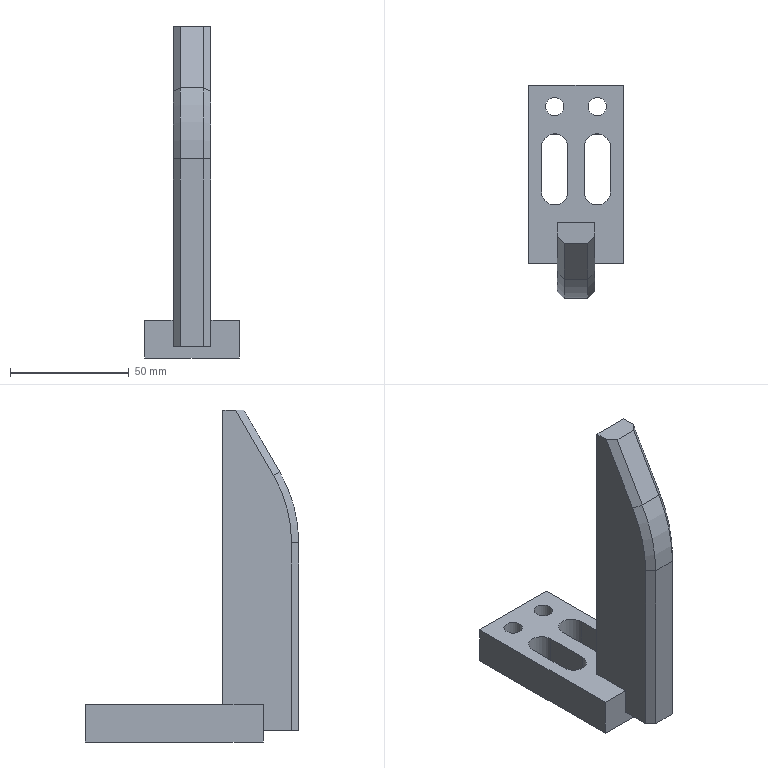Part | NX | features solid 2 | 1 solid | 30 faces | box 40 x 90 x 140 mm | volume 93861 mm3 | plane 21 | cylinder 7 | cone 2 | commonest cylinder face diameters 11 x4 7.8 x2 120 x1
STEP:
#1=CARTESIAN_POINT('',(599.5,194.,-54.));
#2=VERTEX_POINT('',#1);
#3=CARTESIAN_POINT('',(588.5,194.,-54.));
#4=VERTEX_POINT('',#3);
#5=CARTESIAN_POINT('',(594.,194.,-54.));
#6=DIRECTION('',(0.,0.,1.));
#7=DIRECTION('',(0.,-1.,0.));
#8=AXIS2_PLACEMENT_3D('',#5,#6,#7);
#9=CIRCLE('',#8,5.5);
#10=EDGE_CURVE('',#2,#4,#9,.T.);
#11=ORIENTED_EDGE('',*,*,#10,.F.);
#12=CARTESIAN_POINT('',(599.5,175.,-54.));
#13=VERTEX_POINT('',#12);
#14=CARTESIAN_POINT('',(599.5,194.,-54.));
#15=DIRECTION('',(0.,-1.,0.));
#16=VECTOR('',#15,1000.);
#17=LINE('',#14,#16);
#18=EDGE_CURVE('',#2,#13,#17,.T.);
#19=ORIENTED_EDGE('',*,*,#18,.T.);
#20=CARTESIAN_POINT('',(588.5,175.,-54.));
#21=VERTEX_POINT('',#20);
#22=CARTESIAN_POINT('',(594.,175.,-54.));
#23=DIRECTION('',(0.,0.,1.));
#24=DIRECTION('',(0.,-1.,0.));
#25=AXIS2_PLACEMENT_3D('',#22,#23,#24);
#26=CIRCLE('',#25,5.5);
#27=EDGE_CURVE('',#21,#13,#26,.T.);
#28=ORIENTED_EDGE('',*,*,#27,.F.);
#29=CARTESIAN_POINT('',(588.5,194.,-54.));
#30=DIRECTION('',(0.,-1.,0.));
#31=VECTOR('',#30,1000.);
#32=LINE('',#29,#31);
#33=EDGE_CURVE('',#4,#21,#32,.T.);
#34=ORIENTED_EDGE('',*,*,#33,.F.);
#35=EDGE_LOOP('',(#11,#19,#28,#34));
#36=FACE_BOUND('',#35,.T.);
#37=CARTESIAN_POINT('',(576.,207.1,-54.));
#38=VERTEX_POINT('',#37);
#39=CARTESIAN_POINT('',(576.,211.,-54.));
#40=DIRECTION('',(0.,0.,1.));
#41=DIRECTION('',(0.,-1.,0.));
#42=AXIS2_PLACEMENT_3D('',#39,#40,#41);
#43=CIRCLE('',#42,3.9);
#44=EDGE_CURVE('',#38,#38,#43,.T.);
#45=ORIENTED_EDGE('',*,*,#44,.F.);
#46=EDGE_LOOP('',(#45));
#47=FACE_BOUND('',#46,.T.);
#48=CARTESIAN_POINT('',(594.,207.1,-54.));
#49=VERTEX_POINT('',#48);
#50=CARTESIAN_POINT('',(594.,211.,-54.));
#51=DIRECTION('',(0.,0.,1.));
#52=DIRECTION('',(0.,-1.,0.));
#53=AXIS2_PLACEMENT_3D('',#50,#51,#52);
#54=CIRCLE('',#53,3.9);
#55=EDGE_CURVE('',#49,#49,#54,.T.);
#56=ORIENTED_EDGE('',*,*,#55,.F.);
#57=EDGE_LOOP('',(#56));
#58=FACE_BOUND('',#57,.T.);
#59=CARTESIAN_POINT('',(581.5,194.,-54.));
#60=VERTEX_POINT('',#59);
#61=CARTESIAN_POINT('',(581.5,175.,-54.));
#62=VERTEX_POINT('',#61);
#63=CARTESIAN_POINT('',(581.5,194.,-54.));
#64=DIRECTION('',(0.,-1.,0.));
#65=VECTOR('',#64,1000.);
#66=LINE('',#63,#65);
#67=EDGE_CURVE('',#60,#62,#66,.T.);
#68=ORIENTED_EDGE('',*,*,#67,.T.);
#69=CARTESIAN_POINT('',(570.5,175.,-54.));
#70=VERTEX_POINT('',#69);
#71=CARTESIAN_POINT('',(576.,175.,-54.));
#72=DIRECTION('',(0.,0.,1.));
#73=DIRECTION('',(0.,-1.,0.));
#74=AXIS2_PLACEMENT_3D('',#71,#72,#73);
#75=CIRCLE('',#74,5.5);
#76=EDGE_CURVE('',#70,#62,#75,.T.);
#77=ORIENTED_EDGE('',*,*,#76,.F.);
#78=CARTESIAN_POINT('',(570.5,194.,-54.));
#79=VERTEX_POINT('',#78);
#80=CARTESIAN_POINT('',(570.5,194.,-54.));
#81=DIRECTION('',(0.,-1.,0.));
#82=VECTOR('',#81,1000.);
#83=LINE('',#80,#82);
#84=EDGE_CURVE('',#79,#70,#83,.T.);
#85=ORIENTED_EDGE('',*,*,#84,.F.);
#86=CARTESIAN_POINT('',(576.,194.,-54.));
#87=DIRECTION('',(0.,0.,1.));
#88=DIRECTION('',(0.,-1.,0.));
#89=AXIS2_PLACEMENT_3D('',#86,#87,#88);
#90=CIRCLE('',#89,5.5);
#91=EDGE_CURVE('',#60,#79,#90,.T.);
#92=ORIENTED_EDGE('',*,*,#91,.F.);
#93=EDGE_LOOP('',(#68,#77,#85,#92));
#94=FACE_BOUND('',#93,.T.);
#95=CARTESIAN_POINT('',(593.,162.,-54.));
#96=VERTEX_POINT('',#95);
#97=CARTESIAN_POINT('',(577.,162.,-54.));
#98=VERTEX_POINT('',#97);
#99=CARTESIAN_POINT('',(677.,162.,-54.));
#100=DIRECTION('',(-1.,0.,0.));
#101=VECTOR('',#100,1000.);
#102=LINE('',#99,#101);
#103=EDGE_CURVE('',#96,#98,#102,.T.);
#104=ORIENTED_EDGE('',*,*,#103,.F.);
#105=CARTESIAN_POINT('',(593.,145.,-54.));
#106=VERTEX_POINT('',#105);
#107=CARTESIAN_POINT('',(593.,162.,-54.));
#108=DIRECTION('',(0.,1.,0.));
#109=VECTOR('',#108,1000.);
#110=LINE('',#107,#109);
#111=EDGE_CURVE('',#106,#96,#110,.T.);
#112=ORIENTED_EDGE('',*,*,#111,.F.);
#113=CARTESIAN_POINT('',(605.,145.,-54.));
#114=VERTEX_POINT('',#113);
#115=CARTESIAN_POINT('',(585.,145.,-54.));
#116=DIRECTION('',(1.,0.,0.));
#117=VECTOR('',#116,1000.);
#118=LINE('',#115,#117);
#119=EDGE_CURVE('',#106,#114,#118,.T.);
#120=ORIENTED_EDGE('',*,*,#119,.T.);
#121=CARTESIAN_POINT('',(605.,220.,-54.));
#122=VERTEX_POINT('',#121);
#123=CARTESIAN_POINT('',(605.,182.5,-54.));
#124=DIRECTION('',(0.,1.,0.));
#125=VECTOR('',#124,1000.);
#126=LINE('',#123,#125);
#127=EDGE_CURVE('',#114,#122,#126,.T.);
#128=ORIENTED_EDGE('',*,*,#127,.T.);
#129=CARTESIAN_POINT('',(565.,220.,-54.));
#130=VERTEX_POINT('',#129);
#131=CARTESIAN_POINT('',(585.,220.,-54.));
#132=DIRECTION('',(-1.,0.,0.));
#133=VECTOR('',#132,1000.);
#134=LINE('',#131,#133);
#135=EDGE_CURVE('',#122,#130,#134,.T.);
#136=ORIENTED_EDGE('',*,*,#135,.T.);
#137=CARTESIAN_POINT('',(565.,145.,-54.));
#138=VERTEX_POINT('',#137);
#139=CARTESIAN_POINT('',(565.,182.5,-54.));
#140=DIRECTION('',(0.,-1.,0.));
#141=VECTOR('',#140,1000.);
#142=LINE('',#139,#141);
#143=EDGE_CURVE('',#130,#138,#142,.T.);
#144=ORIENTED_EDGE('',*,*,#143,.T.);
#145=CARTESIAN_POINT('',(577.,145.,-54.));
#146=VERTEX_POINT('',#145);
#147=CARTESIAN_POINT('',(585.,145.,-54.));
#148=DIRECTION('',(1.,0.,0.));
#149=VECTOR('',#148,1000.);
#150=LINE('',#147,#149);
#151=EDGE_CURVE('',#138,#146,#150,.T.);
#152=ORIENTED_EDGE('',*,*,#151,.T.);
#153=CARTESIAN_POINT('',(577.,130.,-54.));
#154=DIRECTION('',(0.,1.,0.));
#155=VECTOR('',#154,1000.);
#156=LINE('',#153,#155);
#157=EDGE_CURVE('',#146,#98,#156,.T.);
#158=ORIENTED_EDGE('',*,*,#157,.T.);
#159=EDGE_LOOP('',(#104,#112,#120,#128,#136,#144,#152,#158));
#160=FACE_BOUND('',#159,.T.);
#161=CARTESIAN_POINT('',(585.,182.5,-54.));
#162=DIRECTION('',(0.,0.,1.));
#163=DIRECTION('',(0.,-1.,0.));
#164=AXIS2_PLACEMENT_3D('',#161,#162,#163);
#165=PLANE('',#164);
#166=ADVANCED_FACE('',(#36,#47,#58,#94,#160),#165,.T.);
#167=ORIENTED_EDGE('',*,*,#151,.F.);
#168=CARTESIAN_POINT('',(565.,145.,-70.));
#169=VERTEX_POINT('',#168);
#170=CARTESIAN_POINT('',(565.,145.,-70.));
#171=DIRECTION('',(0.,0.,1.));
#172=VECTOR('',#171,1000.);
#173=LINE('',#170,#172);
#174=EDGE_CURVE('',#169,#138,#173,.T.);
#175=ORIENTED_EDGE('',*,*,#174,.F.);
#176=CARTESIAN_POINT('',(605.,145.,-70.));
#177=VERTEX_POINT('',#176);
#178=CARTESIAN_POINT('',(585.,145.,-70.));
#179=DIRECTION('',(-1.,0.,0.));
#180=VECTOR('',#179,1000.);
#181=LINE('',#178,#180);
#182=EDGE_CURVE('',#177,#169,#181,.T.);
#183=ORIENTED_EDGE('',*,*,#182,.F.);
#184=CARTESIAN_POINT('',(605.,145.,-70.));
#185=DIRECTION('',(0.,0.,1.));
#186=VECTOR('',#185,1000.);
#187=LINE('',#184,#186);
#188=EDGE_CURVE('',#177,#114,#187,.T.);
#189=ORIENTED_EDGE('',*,*,#188,.T.);
#190=ORIENTED_EDGE('',*,*,#119,.F.);
#191=CARTESIAN_POINT('',(593.,145.,-65.));
#192=VERTEX_POINT('',#191);
#193=CARTESIAN_POINT('',(593.,145.,35.));
#194=DIRECTION('',(0.,0.,1.));
#195=VECTOR('',#194,1000.);
#196=LINE('',#193,#195);
#197=EDGE_CURVE('',#192,#106,#196,.T.);
#198=ORIENTED_EDGE('',*,*,#197,.F.);
#199=CARTESIAN_POINT('',(577.,145.,-65.));
#200=VERTEX_POINT('',#199);
#201=CARTESIAN_POINT('',(677.,145.,-65.));
#202=DIRECTION('',(-1.,0.,0.));
#203=VECTOR('',#202,1000.);
#204=LINE('',#201,#203);
#205=EDGE_CURVE('',#192,#200,#204,.T.);
#206=ORIENTED_EDGE('',*,*,#205,.T.);
#207=CARTESIAN_POINT('',(577.,145.,-75.));
#208=DIRECTION('',(0.,0.,1.));
#209=VECTOR('',#208,1000.);
#210=LINE('',#207,#209);
#211=EDGE_CURVE('',#200,#146,#210,.T.);
#212=ORIENTED_EDGE('',*,*,#211,.T.);
#213=EDGE_LOOP('',(#167,#175,#183,#189,#190,#198,#206,#212));
#214=FACE_BOUND('',#213,.T.);
#215=CARTESIAN_POINT('',(585.,145.,-70.));
#216=DIRECTION('',(0.,-1.,0.));
#217=DIRECTION('',(0.,0.,-1.));
#218=AXIS2_PLACEMENT_3D('',#215,#216,#217);
#219=PLANE('',#218);
#220=ADVANCED_FACE('',(#214),#219,.T.);
#221=CARTESIAN_POINT('',(581.5,194.,-70.));
#222=VERTEX_POINT('',#221);
#223=CARTESIAN_POINT('',(581.5,194.,-154.));
#224=DIRECTION('',(0.,0.,1.));
#225=VECTOR('',#224,1000.);
#226=LINE('',#223,#225);
#227=EDGE_CURVE('',#222,#60,#226,.T.);
#228=ORIENTED_EDGE('',*,*,#227,.T.);
#229=ORIENTED_EDGE('',*,*,#91,.T.);
#230=CARTESIAN_POINT('',(570.5,194.,-70.));
#231=VERTEX_POINT('',#230);
#232=CARTESIAN_POINT('',(570.5,194.,-154.));
#233=DIRECTION('',(0.,0.,1.));
#234=VECTOR('',#233,1000.);
#235=LINE('',#232,#234);
#236=EDGE_CURVE('',#231,#79,#235,.T.);
#237=ORIENTED_EDGE('',*,*,#236,.F.);
#238=CARTESIAN_POINT('',(576.,194.,-70.));
#239=DIRECTION('',(0.,0.,1.));
#240=DIRECTION('',(0.,-1.,0.));
#241=AXIS2_PLACEMENT_3D('',#238,#239,#240);
#242=CIRCLE('',#241,5.5);
#243=EDGE_CURVE('',#222,#231,#242,.T.);
#244=ORIENTED_EDGE('',*,*,#243,.F.);
#245=EDGE_LOOP('',(#228,#229,#237,#244));
#246=FACE_BOUND('',#245,.T.);
#247=CARTESIAN_POINT('',(576.,194.,-54.));
#248=DIRECTION('',(0.,0.,-1.));
#249=DIRECTION('',(0.,1.,0.));
#250=AXIS2_PLACEMENT_3D('',#247,#248,#249);
#251=CYLINDRICAL_SURFACE('',#250,5.5);
#252=ADVANCED_FACE('',(#246),#251,.F.);
#253=CARTESIAN_POINT('',(581.5,175.,-70.));
#254=VERTEX_POINT('',#253);
#255=CARTESIAN_POINT('',(581.5,182.5,-70.));
#256=DIRECTION('',(0.,1.,0.));
#257=VECTOR('',#256,1000.);
#258=LINE('',#255,#257);
#259=EDGE_CURVE('',#254,#222,#258,.T.);
#260=ORIENTED_EDGE('',*,*,#259,.T.);
#261=ORIENTED_EDGE('',*,*,#243,.T.);
#262=CARTESIAN_POINT('',(570.5,175.,-70.));
#263=VERTEX_POINT('',#262);
#264=CARTESIAN_POINT('',(570.5,182.5,-70.));
#265=DIRECTION('',(0.,1.,0.));
#266=VECTOR('',#265,1000.);
#267=LINE('',#264,#266);
#268=EDGE_CURVE('',#263,#231,#267,.T.);
#269=ORIENTED_EDGE('',*,*,#268,.F.);
#270=CARTESIAN_POINT('',(576.,175.,-70.));
#271=DIRECTION('',(0.,0.,1.));
#272=DIRECTION('',(0.,-1.,0.));
#273=AXIS2_PLACEMENT_3D('',#270,#271,#272);
#274=CIRCLE('',#273,5.5);
#275=EDGE_CURVE('',#263,#254,#274,.T.);
#276=ORIENTED_EDGE('',*,*,#275,.T.);
#277=EDGE_LOOP('',(#260,#261,#269,#276));
#278=FACE_BOUND('',#277,.T.);
#279=CARTESIAN_POINT('',(565.,220.,-70.));
#280=VERTEX_POINT('',#279);
#281=CARTESIAN_POINT('',(605.,220.,-70.));
#282=VERTEX_POINT('',#281);
#283=CARTESIAN_POINT('',(585.,220.,-70.));
#284=DIRECTION('',(1.,0.,0.));
#285=VECTOR('',#284,1000.);
#286=LINE('',#283,#285);
#287=EDGE_CURVE('',#280,#282,#286,.T.);
#288=ORIENTED_EDGE('',*,*,#287,.T.);
#289=CARTESIAN_POINT('',(605.,182.5,-70.));
#290=DIRECTION('',(0.,-1.,0.));
#291=VECTOR('',#290,1000.);
#292=LINE('',#289,#291);
#293=EDGE_CURVE('',#282,#177,#292,.T.);
#294=ORIENTED_EDGE('',*,*,#293,.T.);
#295=ORIENTED_EDGE('',*,*,#182,.T.);
#296=CARTESIAN_POINT('',(565.,182.5,-70.));
#297=DIRECTION('',(0.,1.,0.));
#298=VECTOR('',#297,1000.);
#299=LINE('',#296,#298);
#300=EDGE_CURVE('',#169,#280,#299,.T.);
#301=ORIENTED_EDGE('',*,*,#300,.T.);
#302=EDGE_LOOP('',(#288,#294,#295,#301));
#303=FACE_BOUND('',#302,.T.);
#304=CARTESIAN_POINT('',(594.,207.1,-70.));
#305=VERTEX_POINT('',#304);
#306=CARTESIAN_POINT('',(594.,211.,-70.));
#307=DIRECTION('',(0.,0.,1.));
#308=DIRECTION('',(0.,-1.,0.));
#309=AXIS2_PLACEMENT_3D('',#306,#307,#308);
#310=CIRCLE('',#309,3.9);
#311=EDGE_CURVE('',#305,#305,#310,.T.);
#312=ORIENTED_EDGE('',*,*,#311,.T.);
#313=EDGE_LOOP('',(#312));
#314=FACE_BOUND('',#313,.T.);
#315=CARTESIAN_POINT('',(576.,207.1,-70.));
#316=VERTEX_POINT('',#315);
#317=CARTESIAN_POINT('',(576.,211.,-70.));
#318=DIRECTION('',(0.,0.,1.));
#319=DIRECTION('',(0.,-1.,0.));
#320=AXIS2_PLACEMENT_3D('',#317,#318,#319);
#321=CIRCLE('',#320,3.9);
#322=EDGE_CURVE('',#316,#316,#321,.T.);
#323=ORIENTED_EDGE('',*,*,#322,.T.);
#324=EDGE_LOOP('',(#323));
#325=FACE_BOUND('',#324,.T.);
#326=CARTESIAN_POINT('',(588.5,175.,-70.));
#327=VERTEX_POINT('',#326);
#328=CARTESIAN_POINT('',(599.5,175.,-70.));
#329=VERTEX_POINT('',#328);
#330=CARTESIAN_POINT('',(594.,175.,-70.));
#331=DIRECTION('',(0.,0.,1.));
#332=DIRECTION('',(0.,-1.,0.));
#333=AXIS2_PLACEMENT_3D('',#330,#331,#332);
#334=CIRCLE('',#333,5.5);
#335=EDGE_CURVE('',#327,#329,#334,.T.);
#336=ORIENTED_EDGE('',*,*,#335,.T.);
#337=CARTESIAN_POINT('',(599.5,194.,-70.));
#338=VERTEX_POINT('',#337);
#339=CARTESIAN_POINT('',(599.5,182.5,-70.));
#340=DIRECTION('',(0.,1.,0.));
#341=VECTOR('',#340,1000.);
#342=LINE('',#339,#341);
#343=EDGE_CURVE('',#329,#338,#342,.T.);
#344=ORIENTED_EDGE('',*,*,#343,.T.);
#345=CARTESIAN_POINT('',(588.5,194.,-70.));
#346=VERTEX_POINT('',#345);
#347=CARTESIAN_POINT('',(594.,194.,-70.));
#348=DIRECTION('',(0.,0.,1.));
#349=DIRECTION('',(0.,-1.,0.));
#350=AXIS2_PLACEMENT_3D('',#347,#348,#349);
#351=CIRCLE('',#350,5.5);
#352=EDGE_CURVE('',#338,#346,#351,.T.);
#353=ORIENTED_EDGE('',*,*,#352,.T.);
#354=CARTESIAN_POINT('',(588.5,182.5,-70.));
#355=DIRECTION('',(0.,1.,0.));
#356=VECTOR('',#355,1000.);
#357=LINE('',#354,#356);
#358=EDGE_CURVE('',#327,#346,#357,.T.);
#359=ORIENTED_EDGE('',*,*,#358,.F.);
#360=EDGE_LOOP('',(#336,#344,#353,#359));
#361=FACE_BOUND('',#360,.T.);
#362=CARTESIAN_POINT('',(585.,182.5,-70.));
#363=DIRECTION('',(0.,0.,-1.));
#364=DIRECTION('',(0.,1.,0.));
#365=AXIS2_PLACEMENT_3D('',#362,#363,#364);
#366=PLANE('',#365);
#367=ADVANCED_FACE('',(#278,#303,#314,#325,#361),#366,.T.);
#368=CARTESIAN_POINT('',(588.5,175.,-154.));
#369=DIRECTION('',(0.,0.,1.));
#370=VECTOR('',#369,1000.);
#371=LINE('',#368,#370);
#372=EDGE_CURVE('',#327,#21,#371,.T.);
#373=ORIENTED_EDGE('',*,*,#372,.T.);
#374=ORIENTED_EDGE('',*,*,#27,.T.);
#375=CARTESIAN_POINT('',(599.5,175.,-154.));
#376=DIRECTION('',(0.,0.,1.));
#377=VECTOR('',#376,1000.);
#378=LINE('',#375,#377);
#379=EDGE_CURVE('',#329,#13,#378,.T.);
#380=ORIENTED_EDGE('',*,*,#379,.F.);
#381=ORIENTED_EDGE('',*,*,#335,.F.);
#382=EDGE_LOOP('',(#373,#374,#380,#381));
#383=FACE_BOUND('',#382,.T.);
#384=CARTESIAN_POINT('',(594.,175.,-54.));
#385=DIRECTION('',(0.,0.,-1.));
#386=DIRECTION('',(0.,1.,0.));
#387=AXIS2_PLACEMENT_3D('',#384,#385,#386);
#388=CYLINDRICAL_SURFACE('',#387,5.5);
#389=ADVANCED_FACE('',(#383),#388,.F.);
#390=CARTESIAN_POINT('',(565.,220.,-70.));
#391=DIRECTION('',(0.,0.,1.));
#392=VECTOR('',#391,1000.);
#393=LINE('',#390,#392);
#394=EDGE_CURVE('',#280,#130,#393,.T.);
#395=ORIENTED_EDGE('',*,*,#394,.F.);
#396=ORIENTED_EDGE('',*,*,#300,.F.);
#397=ORIENTED_EDGE('',*,*,#174,.T.);
#398=ORIENTED_EDGE('',*,*,#143,.F.);
#399=EDGE_LOOP('',(#395,#396,#397,#398));
#400=FACE_BOUND('',#399,.T.);
#401=CARTESIAN_POINT('',(565.,182.5,-70.));
#402=DIRECTION('',(-1.,0.,0.));
#403=DIRECTION('',(0.,0.,1.));
#404=AXIS2_PLACEMENT_3D('',#401,#402,#403);
#405=PLANE('',#404);
#406=ADVANCED_FACE('',(#400),#405,.T.);
#407=ORIENTED_EDGE('',*,*,#188,.F.);
#408=ORIENTED_EDGE('',*,*,#293,.F.);
#409=CARTESIAN_POINT('',(605.,220.,-70.));
#410=DIRECTION('',(0.,0.,1.));
#411=VECTOR('',#410,1000.);
#412=LINE('',#409,#411);
#413=EDGE_CURVE('',#282,#122,#412,.T.);
#414=ORIENTED_EDGE('',*,*,#413,.T.);
#415=ORIENTED_EDGE('',*,*,#127,.F.);
#416=EDGE_LOOP('',(#407,#408,#414,#415));
#417=FACE_BOUND('',#416,.T.);
#418=CARTESIAN_POINT('',(605.,182.5,-70.));
#419=DIRECTION('',(1.,0.,0.));
#420=DIRECTION('',(0.,0.,-1.));
#421=AXIS2_PLACEMENT_3D('',#418,#419,#420);
#422=PLANE('',#421);
#423=ADVANCED_FACE('',(#417),#422,.T.);
#424=ORIENTED_EDGE('',*,*,#287,.F.);
#425=ORIENTED_EDGE('',*,*,#394,.T.);
#426=ORIENTED_EDGE('',*,*,#135,.F.);
#427=ORIENTED_EDGE('',*,*,#413,.F.);
#428=EDGE_LOOP('',(#424,#425,#426,#427));
#429=FACE_BOUND('',#428,.T.);
#430=CARTESIAN_POINT('',(585.,220.,-70.));
#431=DIRECTION('',(0.,1.,0.));
#432=DIRECTION('',(0.,0.,1.));
#433=AXIS2_PLACEMENT_3D('',#430,#431,#432);
#434=PLANE('',#433);
#435=ADVANCED_FACE('',(#429),#434,.T.);
#436=ORIENTED_EDGE('',*,*,#275,.F.);
#437=CARTESIAN_POINT('',(570.5,175.,-154.));
#438=DIRECTION('',(0.,0.,1.));
#439=VECTOR('',#438,1000.);
#440=LINE('',#437,#439);
#441=EDGE_CURVE('',#263,#70,#440,.T.);
#442=ORIENTED_EDGE('',*,*,#441,.T.);
#443=ORIENTED_EDGE('',*,*,#76,.T.);
#444=CARTESIAN_POINT('',(581.5,175.,-154.));
#445=DIRECTION('',(0.,0.,1.));
#446=VECTOR('',#445,1000.);
#447=LINE('',#444,#446);
#448=EDGE_CURVE('',#254,#62,#447,.T.);
#449=ORIENTED_EDGE('',*,*,#448,.F.);
#450=EDGE_LOOP('',(#436,#442,#443,#449));
#451=FACE_BOUND('',#450,.T.);
#452=CARTESIAN_POINT('',(576.,175.,-54.));
#453=DIRECTION('',(0.,0.,-1.));
#454=DIRECTION('',(0.,1.,0.));
#455=AXIS2_PLACEMENT_3D('',#452,#453,#454);
#456=CYLINDRICAL_SURFACE('',#455,5.5);
#457=ADVANCED_FACE('',(#451),#456,.F.);
#458=ORIENTED_EDGE('',*,*,#352,.F.);
#459=CARTESIAN_POINT('',(599.5,194.,-154.));
#460=DIRECTION('',(0.,0.,1.));
#461=VECTOR('',#460,1000.);
#462=LINE('',#459,#461);
#463=EDGE_CURVE('',#338,#2,#462,.T.);
#464=ORIENTED_EDGE('',*,*,#463,.T.);
#465=ORIENTED_EDGE('',*,*,#10,.T.);
#466=CARTESIAN_POINT('',(588.5,194.,-154.));
#467=DIRECTION('',(0.,0.,1.));
#468=VECTOR('',#467,1000.);
#469=LINE('',#466,#468);
#470=EDGE_CURVE('',#346,#4,#469,.T.);
#471=ORIENTED_EDGE('',*,*,#470,.F.);
#472=EDGE_LOOP('',(#458,#464,#465,#471));
#473=FACE_BOUND('',#472,.T.);
#474=CARTESIAN_POINT('',(594.,194.,-54.));
#475=DIRECTION('',(0.,0.,-1.));
#476=DIRECTION('',(0.,1.,0.));
#477=AXIS2_PLACEMENT_3D('',#474,#475,#476);
#478=CYLINDRICAL_SURFACE('',#477,5.5);
#479=ADVANCED_FACE('',(#473),#478,.F.);
#480=ORIENTED_EDGE('',*,*,#311,.F.);
#481=EDGE_LOOP('',(#480));
#482=FACE_BOUND('',#481,.T.);
#483=ORIENTED_EDGE('',*,*,#55,.T.);
#484=EDGE_LOOP('',(#483));
#485=FACE_BOUND('',#484,.T.);
#486=CARTESIAN_POINT('',(594.,211.,-54.));
#487=DIRECTION('',(0.,0.,-1.));
#488=DIRECTION('',(0.,1.,0.));
#489=AXIS2_PLACEMENT_3D('',#486,#487,#488);
#490=CYLINDRICAL_SURFACE('',#489,3.9);
#491=ADVANCED_FACE('',(#482,#485),#490,.F.);
#492=ORIENTED_EDGE('',*,*,#322,.F.);
#493=EDGE_LOOP('',(#492));
#494=FACE_BOUND('',#493,.T.);
#495=ORIENTED_EDGE('',*,*,#44,.T.);
#496=EDGE_LOOP('',(#495));
#497=FACE_BOUND('',#496,.T.);
#498=CARTESIAN_POINT('',(576.,211.,-54.));
#499=DIRECTION('',(0.,0.,-1.));
#500=DIRECTION('',(0.,1.,0.));
#501=AXIS2_PLACEMENT_3D('',#498,#499,#500);
#502=CYLINDRICAL_SURFACE('',#501,3.9);
#503=ADVANCED_FACE('',(#494,#497),#502,.F.);
#504=ORIENTED_EDGE('',*,*,#343,.F.);
#505=ORIENTED_EDGE('',*,*,#379,.T.);
#506=ORIENTED_EDGE('',*,*,#18,.F.);
#507=ORIENTED_EDGE('',*,*,#463,.F.);
#508=EDGE_LOOP('',(#504,#505,#506,#507));
#509=FACE_BOUND('',#508,.T.);
#510=CARTESIAN_POINT('',(599.5,194.,-154.));
#511=DIRECTION('',(1.,0.,0.));
#512=DIRECTION('',(0.,0.,-1.));
#513=AXIS2_PLACEMENT_3D('',#510,#511,#512);
#514=PLANE('',#513);
#515=ADVANCED_FACE('',(#509),#514,.F.);
#516=ORIENTED_EDGE('',*,*,#372,.F.);
#517=ORIENTED_EDGE('',*,*,#358,.T.);
#518=ORIENTED_EDGE('',*,*,#470,.T.);
#519=ORIENTED_EDGE('',*,*,#33,.T.);
#520=EDGE_LOOP('',(#516,#517,#518,#519));
#521=FACE_BOUND('',#520,.T.);
#522=CARTESIAN_POINT('',(588.5,194.,-154.));
#523=DIRECTION('',(1.,0.,0.));
#524=DIRECTION('',(0.,0.,-1.));
#525=AXIS2_PLACEMENT_3D('',#522,#523,#524);
#526=PLANE('',#525);
#527=ADVANCED_FACE('',(#521),#526,.T.);
#528=ORIENTED_EDGE('',*,*,#441,.F.);
#529=ORIENTED_EDGE('',*,*,#268,.T.);
#530=ORIENTED_EDGE('',*,*,#236,.T.);
#531=ORIENTED_EDGE('',*,*,#84,.T.);
#532=EDGE_LOOP('',(#528,#529,#530,#531));
#533=FACE_BOUND('',#532,.T.);
#534=CARTESIAN_POINT('',(570.5,194.,-154.));
#535=DIRECTION('',(1.,0.,0.));
#536=DIRECTION('',(0.,0.,-1.));
#537=AXIS2_PLACEMENT_3D('',#534,#535,#536);
#538=PLANE('',#537);
#539=ADVANCED_FACE('',(#533),#538,.T.);
#540=ORIENTED_EDGE('',*,*,#259,.F.);
#541=ORIENTED_EDGE('',*,*,#448,.T.);
#542=ORIENTED_EDGE('',*,*,#67,.F.);
#543=ORIENTED_EDGE('',*,*,#227,.F.);
#544=EDGE_LOOP('',(#540,#541,#542,#543));
#545=FACE_BOUND('',#544,.T.);
#546=CARTESIAN_POINT('',(581.5,194.,-154.));
#547=DIRECTION('',(1.,0.,0.));
#548=DIRECTION('',(0.,0.,-1.));
#549=AXIS2_PLACEMENT_3D('',#546,#547,#548);
#550=PLANE('',#549);
#551=ADVANCED_FACE('',(#545),#550,.F.);
#552=ORIENTED_EDGE('',*,*,#211,.F.);
#553=CARTESIAN_POINT('',(577.,133.,-65.));
#554=VERTEX_POINT('',#553);
#555=CARTESIAN_POINT('',(577.,130.,-65.));
#556=DIRECTION('',(0.,1.,0.));
#557=VECTOR('',#556,1000.);
#558=LINE('',#555,#557);
#559=EDGE_CURVE('',#554,#200,#558,.T.);
#560=ORIENTED_EDGE('',*,*,#559,.F.);
#561=CARTESIAN_POINT('',(577.,133.,13.923));
#562=VERTEX_POINT('',#561);
#563=CARTESIAN_POINT('',(577.,133.,35.));
#564=DIRECTION('',(0.,0.,-1.));
#565=VECTOR('',#564,1000.);
#566=LINE('',#563,#565);
#567=EDGE_CURVE('',#562,#554,#566,.T.);
#568=ORIENTED_EDGE('',*,*,#567,.F.);
#569=CARTESIAN_POINT('',(577.,140.637,42.423));
#570=VERTEX_POINT('',#569);
#571=CARTESIAN_POINT('',(577.,190.,13.923));
#572=DIRECTION('',(1.,0.,0.));
#573=DIRECTION('',(0.,0.,1.));
#574=AXIS2_PLACEMENT_3D('',#571,#572,#573);
#575=CIRCLE('',#574,57.);
#576=EDGE_CURVE('',#570,#562,#575,.T.);
#577=ORIENTED_EDGE('',*,*,#576,.F.);
#578=CARTESIAN_POINT('',(577.,156.558,70.));
#579=VERTEX_POINT('',#578);
#580=CARTESIAN_POINT('',(577.,149.919,58.5));
#581=DIRECTION('',(0.,-0.5,-0.866));
#582=VECTOR('',#581,1000.);
#583=LINE('',#580,#582);
#584=EDGE_CURVE('',#579,#570,#583,.T.);
#585=ORIENTED_EDGE('',*,*,#584,.F.);
#586=CARTESIAN_POINT('',(577.,162.,70.));
#587=VERTEX_POINT('',#586);
#588=CARTESIAN_POINT('',(577.,130.,70.));
#589=DIRECTION('',(0.,1.,0.));
#590=VECTOR('',#589,1000.);
#591=LINE('',#588,#590);
#592=EDGE_CURVE('',#579,#587,#591,.T.);
#593=ORIENTED_EDGE('',*,*,#592,.T.);
#594=CARTESIAN_POINT('',(577.,162.,35.));
#595=DIRECTION('',(0.,0.,-1.));
#596=VECTOR('',#595,1000.);
#597=LINE('',#594,#596);
#598=EDGE_CURVE('',#587,#98,#597,.T.);
#599=ORIENTED_EDGE('',*,*,#598,.T.);
#600=ORIENTED_EDGE('',*,*,#157,.F.);
#601=EDGE_LOOP('',(#552,#560,#568,#577,#585,#593,#599,#600));
#602=FACE_BOUND('',#601,.T.);
#603=CARTESIAN_POINT('',(577.,130.,35.));
#604=DIRECTION('',(1.,0.,0.));
#605=DIRECTION('',(0.,0.,-1.));
#606=AXIS2_PLACEMENT_3D('',#603,#604,#605);
#607=PLANE('',#606);
#608=ADVANCED_FACE('',(#602),#607,.F.);
#609=ORIENTED_EDGE('',*,*,#103,.T.);
#610=ORIENTED_EDGE('',*,*,#598,.F.);
#611=CARTESIAN_POINT('',(593.,162.,70.));
#612=VERTEX_POINT('',#611);
#613=CARTESIAN_POINT('',(577.,162.,70.));
#614=DIRECTION('',(1.,0.,0.));
#615=VECTOR('',#614,1000.);
#616=LINE('',#613,#615);
#617=EDGE_CURVE('',#587,#612,#616,.T.);
#618=ORIENTED_EDGE('',*,*,#617,.T.);
#619=CARTESIAN_POINT('',(593.,162.,35.));
#620=DIRECTION('',(0.,0.,-1.));
#621=VECTOR('',#620,1000.);
#622=LINE('',#619,#621);
#623=EDGE_CURVE('',#612,#96,#622,.T.);
#624=ORIENTED_EDGE('',*,*,#623,.T.);
#625=EDGE_LOOP('',(#609,#610,#618,#624));
#626=FACE_BOUND('',#625,.T.);
#627=CARTESIAN_POINT('',(577.,162.,35.));
#628=DIRECTION('',(0.,-1.,0.));
#629=DIRECTION('',(0.,0.,-1.));
#630=AXIS2_PLACEMENT_3D('',#627,#628,#629);
#631=PLANE('',#630);
#632=ADVANCED_FACE('',(#626),#631,.F.);
#633=ORIENTED_EDGE('',*,*,#197,.T.);
#634=ORIENTED_EDGE('',*,*,#111,.T.);
#635=ORIENTED_EDGE('',*,*,#623,.F.);
#636=CARTESIAN_POINT('',(593.,156.558,70.));
#637=VERTEX_POINT('',#636);
#638=CARTESIAN_POINT('',(593.,162.,70.));
#639=DIRECTION('',(0.,-1.,0.));
#640=VECTOR('',#639,1000.);
#641=LINE('',#638,#640);
#642=EDGE_CURVE('',#612,#637,#641,.T.);
#643=ORIENTED_EDGE('',*,*,#642,.T.);
#644=CARTESIAN_POINT('',(593.,140.637,42.423));
#645=VERTEX_POINT('',#644);
#646=CARTESIAN_POINT('',(593.,157.919,72.356));
#647=DIRECTION('',(0.,0.5,0.866));
#648=VECTOR('',#647,1000.);
#649=LINE('',#646,#648);
#650=EDGE_CURVE('',#645,#637,#649,.T.);
#651=ORIENTED_EDGE('',*,*,#650,.F.);
#652=CARTESIAN_POINT('',(593.,133.,13.923));
#653=VERTEX_POINT('',#652);
#654=CARTESIAN_POINT('',(593.,190.,13.923));
#655=DIRECTION('',(-1.,0.,0.));
#656=DIRECTION('',(0.,0.,-1.));
#657=AXIS2_PLACEMENT_3D('',#654,#655,#656);
#658=CIRCLE('',#657,57.);
#659=EDGE_CURVE('',#653,#645,#658,.T.);
#660=ORIENTED_EDGE('',*,*,#659,.F.);
#661=CARTESIAN_POINT('',(593.,133.,-65.));
#662=VERTEX_POINT('',#661);
#663=CARTESIAN_POINT('',(593.,133.,35.));
#664=DIRECTION('',(0.,0.,1.));
#665=VECTOR('',#664,1000.);
#666=LINE('',#663,#665);
#667=EDGE_CURVE('',#662,#653,#666,.T.);
#668=ORIENTED_EDGE('',*,*,#667,.F.);
#669=CARTESIAN_POINT('',(593.,162.,-65.));
#670=DIRECTION('',(0.,-1.,0.));
#671=VECTOR('',#670,1000.);
#672=LINE('',#669,#671);
#673=EDGE_CURVE('',#192,#662,#672,.T.);
#674=ORIENTED_EDGE('',*,*,#673,.F.);
#675=EDGE_LOOP('',(#633,#634,#635,#643,#651,#660,#668,#674));
#676=FACE_BOUND('',#675,.T.);
#677=CARTESIAN_POINT('',(593.,162.,35.));
#678=DIRECTION('',(-1.,0.,0.));
#679=DIRECTION('',(0.,0.,1.));
#680=AXIS2_PLACEMENT_3D('',#677,#678,#679);
#681=PLANE('',#680);
#682=ADVANCED_FACE('',(#676),#681,.F.);
#683=ORIENTED_EDGE('',*,*,#205,.F.);
#684=ORIENTED_EDGE('',*,*,#673,.T.);
#685=CARTESIAN_POINT('',(590.,130.,-65.));
#686=VERTEX_POINT('',#685);
#687=CARTESIAN_POINT('',(590.,130.,-65.));
#688=DIRECTION('',(0.7071,0.7071,0.));
#689=VECTOR('',#688,1000.);
#690=LINE('',#687,#689);
#691=EDGE_CURVE('',#686,#662,#690,.T.);
#692=ORIENTED_EDGE('',*,*,#691,.F.);
#693=CARTESIAN_POINT('',(580.,130.,-65.));
#694=VERTEX_POINT('',#693);
#695=CARTESIAN_POINT('',(593.,130.,-65.));
#696=DIRECTION('',(-1.,0.,0.));
#697=VECTOR('',#696,1000.);
#698=LINE('',#695,#697);
#699=EDGE_CURVE('',#686,#694,#698,.T.);
#700=ORIENTED_EDGE('',*,*,#699,.T.);
#701=CARTESIAN_POINT('',(577.,133.,-65.));
#702=DIRECTION('',(0.7071,-0.7071,0.));
#703=VECTOR('',#702,1000.);
#704=LINE('',#701,#703);
#705=EDGE_CURVE('',#554,#694,#704,.T.);
#706=ORIENTED_EDGE('',*,*,#705,.F.);
#707=ORIENTED_EDGE('',*,*,#559,.T.);
#708=EDGE_LOOP('',(#683,#684,#692,#700,#706,#707));
#709=FACE_BOUND('',#708,.T.);
#710=CARTESIAN_POINT('',(577.,130.,-65.));
#711=DIRECTION('',(0.,0.,1.));
#712=DIRECTION('',(0.,-1.,0.));
#713=AXIS2_PLACEMENT_3D('',#710,#711,#712);
#714=PLANE('',#713);
#715=ADVANCED_FACE('',(#709),#714,.F.);
#716=CARTESIAN_POINT('',(580.,130.,13.923));
#717=VERTEX_POINT('',#716);
#718=CARTESIAN_POINT('',(590.,130.,13.923));
#719=VERTEX_POINT('',#718);
#720=CARTESIAN_POINT('',(593.,130.,13.923));
#721=DIRECTION('',(1.,0.,0.));
#722=VECTOR('',#721,1000.);
#723=LINE('',#720,#722);
#724=EDGE_CURVE('',#717,#719,#723,.T.);
#725=ORIENTED_EDGE('',*,*,#724,.F.);
#726=CARTESIAN_POINT('',(580.,130.,35.));
#727=DIRECTION('',(0.,0.,1.));
#728=VECTOR('',#727,1000.);
#729=LINE('',#726,#728);
#730=EDGE_CURVE('',#694,#717,#729,.T.);
#731=ORIENTED_EDGE('',*,*,#730,.F.);
#732=ORIENTED_EDGE('',*,*,#699,.F.);
#733=CARTESIAN_POINT('',(590.,130.,35.));
#734=DIRECTION('',(0.,0.,-1.));
#735=VECTOR('',#734,1000.);
#736=LINE('',#733,#735);
#737=EDGE_CURVE('',#719,#686,#736,.T.);
#738=ORIENTED_EDGE('',*,*,#737,.F.);
#739=EDGE_LOOP('',(#725,#731,#732,#738));
#740=FACE_BOUND('',#739,.T.);
#741=CARTESIAN_POINT('',(593.,130.,35.));
#742=DIRECTION('',(0.,1.,0.));
#743=DIRECTION('',(0.,0.,1.));
#744=AXIS2_PLACEMENT_3D('',#741,#742,#743);
#745=PLANE('',#744);
#746=ADVANCED_FACE('',(#740),#745,.F.);
#747=ORIENTED_EDGE('',*,*,#642,.F.);
#748=ORIENTED_EDGE('',*,*,#617,.F.);
#749=ORIENTED_EDGE('',*,*,#592,.F.);
#750=CARTESIAN_POINT('',(580.,153.094,70.));
#751=VERTEX_POINT('',#750);
#752=CARTESIAN_POINT('',(590.143,141.382,70.));
#753=DIRECTION('',(-0.6547,0.7559,0.));
#754=VECTOR('',#753,1000.);
#755=LINE('',#752,#754);
#756=EDGE_CURVE('',#751,#579,#755,.T.);
#757=ORIENTED_EDGE('',*,*,#756,.F.);
#758=CARTESIAN_POINT('',(590.,153.094,70.));
#759=VERTEX_POINT('',#758);
#760=CARTESIAN_POINT('',(677.,153.094,70.));
#761=DIRECTION('',(-1.,0.,0.));
#762=VECTOR('',#761,1000.);
#763=LINE('',#760,#762);
#764=EDGE_CURVE('',#759,#751,#763,.T.);
#765=ORIENTED_EDGE('',*,*,#764,.F.);
#766=CARTESIAN_POINT('',(573.,133.464,70.));
#767=DIRECTION('',(-0.6547,-0.7559,0.));
#768=VECTOR('',#767,1000.);
#769=LINE('',#766,#768);
#770=EDGE_CURVE('',#637,#759,#769,.T.);
#771=ORIENTED_EDGE('',*,*,#770,.F.);
#772=EDGE_LOOP('',(#747,#748,#749,#757,#765,#771));
#773=FACE_BOUND('',#772,.T.);
#774=CARTESIAN_POINT('',(577.,130.,70.));
#775=DIRECTION('',(0.,0.,1.));
#776=DIRECTION('',(0.,-1.,0.));
#777=AXIS2_PLACEMENT_3D('',#774,#775,#776);
#778=PLANE('',#777);
#779=ADVANCED_FACE('',(#773),#778,.T.);
#780=ORIENTED_EDGE('',*,*,#764,.T.);
#781=CARTESIAN_POINT('',(580.,138.038,43.923));
#782=VERTEX_POINT('',#781);
#783=CARTESIAN_POINT('',(580.,130.,30.));
#784=DIRECTION('',(0.,0.5,0.866));
#785=VECTOR('',#784,1000.);
#786=LINE('',#783,#785);
#787=EDGE_CURVE('',#782,#751,#786,.T.);
#788=ORIENTED_EDGE('',*,*,#787,.F.);
#789=CARTESIAN_POINT('',(590.,138.038,43.923));
#790=VERTEX_POINT('',#789);
#791=CARTESIAN_POINT('',(677.,138.038,43.923));
#792=DIRECTION('',(-1.,0.,0.));
#793=VECTOR('',#792,1000.);
#794=LINE('',#791,#793);
#795=EDGE_CURVE('',#790,#782,#794,.T.);
#796=ORIENTED_EDGE('',*,*,#795,.F.);
#797=CARTESIAN_POINT('',(590.,130.,30.));
#798=DIRECTION('',(0.,-0.5,-0.866));
#799=VECTOR('',#798,1000.);
#800=LINE('',#797,#799);
#801=EDGE_CURVE('',#759,#790,#800,.T.);
#802=ORIENTED_EDGE('',*,*,#801,.F.);
#803=EDGE_LOOP('',(#780,#788,#796,#802));
#804=FACE_BOUND('',#803,.T.);
#805=CARTESIAN_POINT('',(677.,130.,30.));
#806=DIRECTION('',(0.,0.866,-0.5));
#807=DIRECTION('',(0.,0.5,0.866));
#808=AXIS2_PLACEMENT_3D('',#805,#806,#807);
#809=PLANE('',#808);
#810=ADVANCED_FACE('',(#804),#809,.F.);
#811=ORIENTED_EDGE('',*,*,#724,.T.);
#812=CARTESIAN_POINT('',(590.,190.,13.923));
#813=DIRECTION('',(1.,0.,0.));
#814=DIRECTION('',(0.,0.,-1.));
#815=AXIS2_PLACEMENT_3D('',#812,#813,#814);
#816=CIRCLE('',#815,60.);
#817=EDGE_CURVE('',#790,#719,#816,.T.);
#818=ORIENTED_EDGE('',*,*,#817,.F.);
#819=ORIENTED_EDGE('',*,*,#795,.T.);
#820=CARTESIAN_POINT('',(580.,190.,13.923));
#821=DIRECTION('',(-1.,0.,0.));
#822=DIRECTION('',(0.,0.,1.));
#823=AXIS2_PLACEMENT_3D('',#820,#821,#822);
#824=CIRCLE('',#823,60.);
#825=EDGE_CURVE('',#717,#782,#824,.T.);
#826=ORIENTED_EDGE('',*,*,#825,.F.);
#827=EDGE_LOOP('',(#811,#818,#819,#826));
#828=FACE_BOUND('',#827,.T.);
#829=CARTESIAN_POINT('',(677.,190.,13.923));
#830=DIRECTION('',(-1.,0.,0.));
#831=DIRECTION('',(0.,0.,1.));
#832=AXIS2_PLACEMENT_3D('',#829,#830,#831);
#833=CYLINDRICAL_SURFACE('',#832,60.);
#834=ADVANCED_FACE('',(#828),#833,.T.);
#835=ORIENTED_EDGE('',*,*,#770,.T.);
#836=ORIENTED_EDGE('',*,*,#801,.T.);
#837=CARTESIAN_POINT('',(590.,138.038,43.923));
#838=DIRECTION('',(0.7071,0.6124,-0.3536));
#839=VECTOR('',#838,1000.);
#840=LINE('',#837,#839);
#841=EDGE_CURVE('',#790,#645,#840,.T.);
#842=ORIENTED_EDGE('',*,*,#841,.T.);
#843=ORIENTED_EDGE('',*,*,#650,.T.);
#844=EDGE_LOOP('',(#835,#836,#842,#843));
#845=FACE_BOUND('',#844,.T.);
#846=CARTESIAN_POINT('',(593.,157.919,72.356));
#847=DIRECTION('',(-0.7071,0.6124,-0.3536));
#848=DIRECTION('',(-0.6547,-0.7559,0.));
#849=AXIS2_PLACEMENT_3D('',#846,#847,#848);
#850=PLANE('',#849);
#851=ADVANCED_FACE('',(#845),#850,.F.);
#852=ORIENTED_EDGE('',*,*,#841,.F.);
#853=ORIENTED_EDGE('',*,*,#817,.T.);
#854=CARTESIAN_POINT('',(621.5,161.5,13.923));
#855=DIRECTION('',(0.7071,0.7071,0.));
#856=VECTOR('',#855,1000.);
#857=LINE('',#854,#856);
#858=EDGE_CURVE('',#719,#653,#857,.T.);
#859=ORIENTED_EDGE('',*,*,#858,.T.);
#860=ORIENTED_EDGE('',*,*,#659,.T.);
#861=EDGE_LOOP('',(#852,#853,#859,#860));
#862=FACE_BOUND('',#861,.T.);
#863=CARTESIAN_POINT('',(593.,190.,13.923));
#864=DIRECTION('',(-1.,0.,0.));
#865=DIRECTION('',(0.,0.,1.));
#866=AXIS2_PLACEMENT_3D('',#863,#864,#865);
#867=CONICAL_SURFACE('',#866,57.,0.7854);
#868=ADVANCED_FACE('',(#862),#867,.T.);
#869=ORIENTED_EDGE('',*,*,#858,.F.);
#870=ORIENTED_EDGE('',*,*,#737,.T.);
#871=ORIENTED_EDGE('',*,*,#691,.T.);
#872=ORIENTED_EDGE('',*,*,#667,.T.);
#873=EDGE_LOOP('',(#869,#870,#871,#872));
#874=FACE_BOUND('',#873,.T.);
#875=CARTESIAN_POINT('',(590.,130.,35.));
#876=DIRECTION('',(-0.7071,0.7071,0.));
#877=DIRECTION('',(-0.7071,-0.7071,0.));
#878=AXIS2_PLACEMENT_3D('',#875,#876,#877);
#879=PLANE('',#878);
#880=ADVANCED_FACE('',(#874),#879,.F.);
#881=ORIENTED_EDGE('',*,*,#756,.T.);
#882=ORIENTED_EDGE('',*,*,#584,.T.);
#883=CARTESIAN_POINT('',(577.,140.637,42.423));
#884=DIRECTION('',(0.7071,-0.6124,0.3536));
#885=VECTOR('',#884,1000.);
#886=LINE('',#883,#885);
#887=EDGE_CURVE('',#570,#782,#886,.T.);
#888=ORIENTED_EDGE('',*,*,#887,.T.);
#889=ORIENTED_EDGE('',*,*,#787,.T.);
#890=EDGE_LOOP('',(#881,#882,#888,#889));
#891=FACE_BOUND('',#890,.T.);
#892=CARTESIAN_POINT('',(580.,130.,30.));
#893=DIRECTION('',(0.7071,0.6124,-0.3536));
#894=DIRECTION('',(-0.6547,0.7559,0.));
#895=AXIS2_PLACEMENT_3D('',#892,#893,#894);
#896=PLANE('',#895);
#897=ADVANCED_FACE('',(#891),#896,.F.);
#898=ORIENTED_EDGE('',*,*,#887,.F.);
#899=ORIENTED_EDGE('',*,*,#576,.T.);
#900=CARTESIAN_POINT('',(548.5,161.5,13.923));
#901=DIRECTION('',(0.7071,-0.7071,0.));
#902=VECTOR('',#901,1000.);
#903=LINE('',#900,#902);
#904=EDGE_CURVE('',#562,#717,#903,.T.);
#905=ORIENTED_EDGE('',*,*,#904,.T.);
#906=ORIENTED_EDGE('',*,*,#825,.T.);
#907=EDGE_LOOP('',(#898,#899,#905,#906));
#908=FACE_BOUND('',#907,.T.);
#909=CARTESIAN_POINT('',(577.,190.,13.923));
#910=DIRECTION('',(1.,0.,0.));
#911=DIRECTION('',(0.,0.,-1.));
#912=AXIS2_PLACEMENT_3D('',#909,#910,#911);
#913=CONICAL_SURFACE('',#912,57.,0.7854);
#914=ADVANCED_FACE('',(#908),#913,.T.);
#915=ORIENTED_EDGE('',*,*,#904,.F.);
#916=ORIENTED_EDGE('',*,*,#567,.T.);
#917=ORIENTED_EDGE('',*,*,#705,.T.);
#918=ORIENTED_EDGE('',*,*,#730,.T.);
#919=EDGE_LOOP('',(#915,#916,#917,#918));
#920=FACE_BOUND('',#919,.T.);
#921=CARTESIAN_POINT('',(577.,133.,35.));
#922=DIRECTION('',(0.7071,0.7071,0.));
#923=DIRECTION('',(-0.7071,0.7071,0.));
#924=AXIS2_PLACEMENT_3D('',#921,#922,#923);
#925=PLANE('',#924);
#926=ADVANCED_FACE('',(#920),#925,.F.);
#927=CLOSED_SHELL('',(#166,#220,#252,#367,#389,#406,#423,#435,#457,#479,#491,#503,#515,#527,#539,#551,#608,#632,#682,#715,#746,#779,#810,#834,#851,#868,#880,#897,#914,#926));
#928=MANIFOLD_SOLID_BREP('',#927);
#929=(LENGTH_UNIT()NAMED_UNIT(*)SI_UNIT(.MILLI.,.METRE.));
#930=UNCERTAINTY_MEASURE_WITH_UNIT(LENGTH_MEASURE(0.00001),#929,'','');
#931=(NAMED_UNIT(*)PLANE_ANGLE_UNIT()SI_UNIT($,.RADIAN.));
#932=(NAMED_UNIT(*)SI_UNIT($,.STERADIAN.)SOLID_ANGLE_UNIT());
#933=(GEOMETRIC_REPRESENTATION_CONTEXT(3)GLOBAL_UNCERTAINTY_ASSIGNED_CONTEXT((#930))GLOBAL_UNIT_ASSIGNED_CONTEXT((#929,#931,#932))REPRESENTATION_CONTEXT('',''));
#934=ADVANCED_BREP_SHAPE_REPRESENTATION('',(#928),#933);